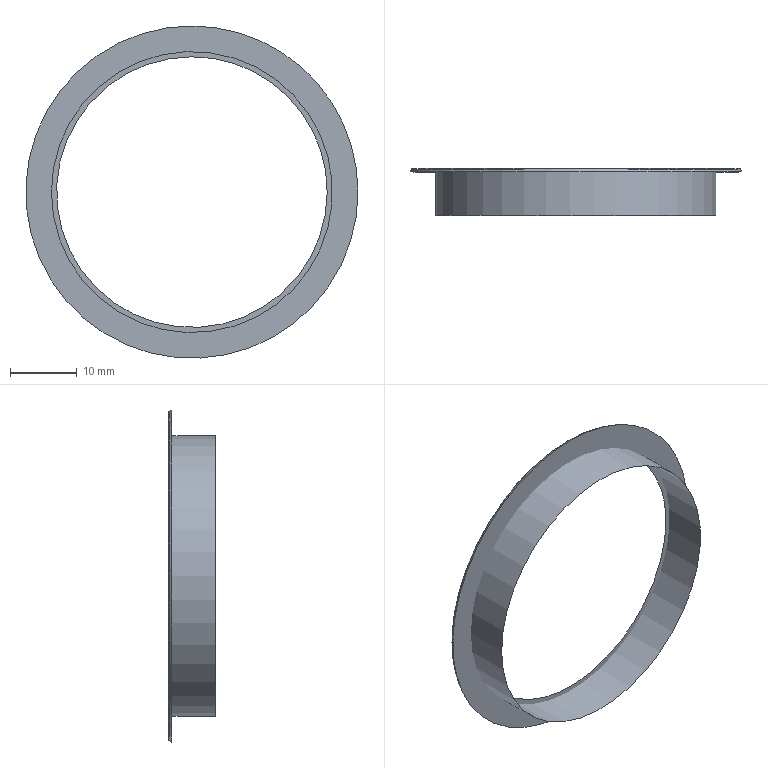Part | STEP file | P1211200001_D | 1 solid | 6 faces | box 49.654 x 7 x 49.654 mm | volume 6705 mm3 | plane 2 | cone 2 | cylinder 1 | torus 1 | commonest cylinder face diameters 42 x1